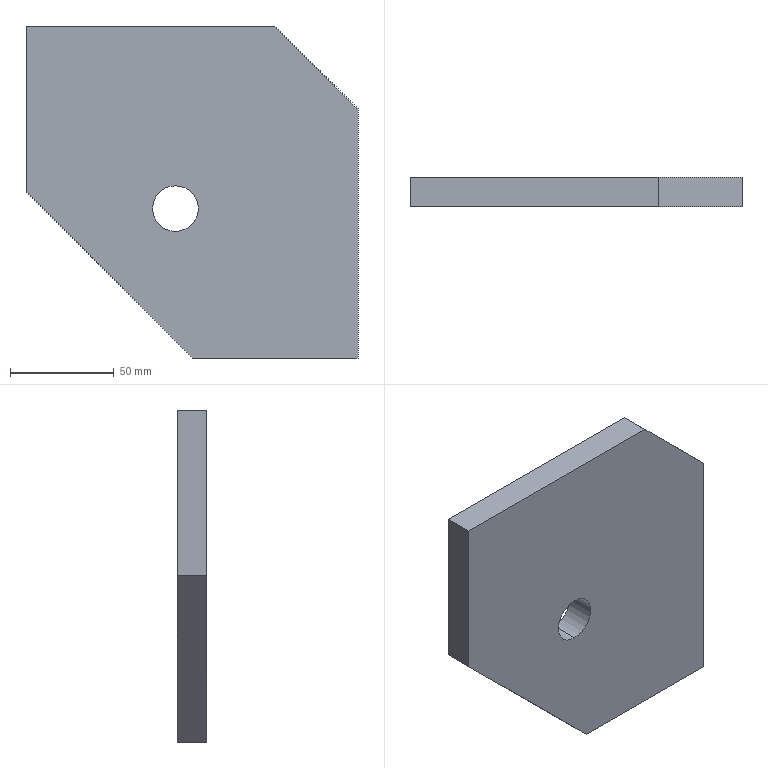Part | SolidWorks | features ICE 2, BaseBody 1 | 1 solid | 10 faces | box 160 x 14 x 160 mm | volume 297078 mm3 | plane 8 | cylinder 2 | commonest cylinder face diameters 22 x2
STEP:
#1=CARTESIAN_POINT('',(-88.,0.,-99.));
#2=VERTEX_POINT('',#1);
#3=CARTESIAN_POINT('',(-88.,0.,-77.));
#4=VERTEX_POINT('',#3);
#5=CARTESIAN_POINT('',(-88.,0.,-88.));
#6=DIRECTION('',(0.,1.,0.));
#7=DIRECTION('',(0.,0.,1.));
#8=AXIS2_PLACEMENT_3D('',#5,#6,#7);
#9=CIRCLE('',#8,11.);
#10=EDGE_CURVE('',#2,#4,#9,.T.);
#11=ORIENTED_EDGE('',*,*,#10,.F.);
#12=CARTESIAN_POINT('',(-88.,14.,-99.));
#13=VERTEX_POINT('',#12);
#14=CARTESIAN_POINT('',(-88.,0.,-99.));
#15=DIRECTION('',(0.,1.,0.));
#16=VECTOR('',#15,1000.);
#17=LINE('',#14,#16);
#18=EDGE_CURVE('',#2,#13,#17,.T.);
#19=ORIENTED_EDGE('',*,*,#18,.T.);
#20=CARTESIAN_POINT('',(-88.,14.,-77.));
#21=VERTEX_POINT('',#20);
#22=CARTESIAN_POINT('',(-88.,14.,-88.));
#23=DIRECTION('',(0.,1.,0.));
#24=DIRECTION('',(0.,0.,1.));
#25=AXIS2_PLACEMENT_3D('',#22,#23,#24);
#26=CIRCLE('',#25,11.);
#27=EDGE_CURVE('',#13,#21,#26,.T.);
#28=ORIENTED_EDGE('',*,*,#27,.T.);
#29=CARTESIAN_POINT('',(-88.,0.,-77.));
#30=DIRECTION('',(0.,1.,0.));
#31=VECTOR('',#30,1000.);
#32=LINE('',#29,#31);
#33=EDGE_CURVE('',#4,#21,#32,.T.);
#34=ORIENTED_EDGE('',*,*,#33,.F.);
#35=EDGE_LOOP('',(#11,#19,#28,#34));
#36=FACE_OUTER_BOUND('',#35,.T.);
#37=CARTESIAN_POINT('',(-88.,0.,-88.));
#38=DIRECTION('',(0.,1.,0.));
#39=DIRECTION('',(0.,0.,1.));
#40=AXIS2_PLACEMENT_3D('',#37,#38,#39);
#41=CYLINDRICAL_SURFACE('',#40,11.);
#42=ADVANCED_FACE('',(#36),#41,.F.);
#43=CARTESIAN_POINT('',(-160.,14.,0.));
#44=VERTEX_POINT('',#43);
#45=CARTESIAN_POINT('',(-160.,14.,-80.));
#46=VERTEX_POINT('',#45);
#47=CARTESIAN_POINT('',(-160.,14.,0.));
#48=DIRECTION('',(0.,0.,-1.));
#49=VECTOR('',#48,1000.);
#50=LINE('',#47,#49);
#51=EDGE_CURVE('',#44,#46,#50,.T.);
#52=ORIENTED_EDGE('',*,*,#51,.F.);
#53=CARTESIAN_POINT('',(-40.,14.,0.));
#54=VERTEX_POINT('',#53);
#55=CARTESIAN_POINT('',(0.,14.,0.));
#56=DIRECTION('',(1.,0.,0.));
#57=VECTOR('',#56,1000.);
#58=LINE('',#55,#57);
#59=EDGE_CURVE('',#44,#54,#58,.T.);
#60=ORIENTED_EDGE('',*,*,#59,.T.);
#61=CARTESIAN_POINT('',(0.,14.,-40.));
#62=VERTEX_POINT('',#61);
#63=CARTESIAN_POINT('',(-40.,14.,0.));
#64=DIRECTION('',(0.7071,0.,-0.7071));
#65=VECTOR('',#64,1000.);
#66=LINE('',#63,#65);
#67=EDGE_CURVE('',#54,#62,#66,.T.);
#68=ORIENTED_EDGE('',*,*,#67,.T.);
#69=CARTESIAN_POINT('',(0.,14.,-160.));
#70=VERTEX_POINT('',#69);
#71=CARTESIAN_POINT('',(0.,14.,0.));
#72=DIRECTION('',(0.,0.,-1.));
#73=VECTOR('',#72,1000.);
#74=LINE('',#71,#73);
#75=EDGE_CURVE('',#62,#70,#74,.T.);
#76=ORIENTED_EDGE('',*,*,#75,.T.);
#77=CARTESIAN_POINT('',(-80.,14.,-160.));
#78=VERTEX_POINT('',#77);
#79=CARTESIAN_POINT('',(0.,14.,-160.));
#80=DIRECTION('',(1.,0.,0.));
#81=VECTOR('',#80,1000.);
#82=LINE('',#79,#81);
#83=EDGE_CURVE('',#78,#70,#82,.T.);
#84=ORIENTED_EDGE('',*,*,#83,.F.);
#85=CARTESIAN_POINT('',(-40.,14.,-200.));
#86=DIRECTION('',(-0.7071,0.,0.7071));
#87=VECTOR('',#86,1000.);
#88=LINE('',#85,#87);
#89=EDGE_CURVE('',#78,#46,#88,.T.);
#90=ORIENTED_EDGE('',*,*,#89,.T.);
#91=EDGE_LOOP('',(#52,#60,#68,#76,#84,#90));
#92=FACE_OUTER_BOUND('',#91,.T.);
#93=CARTESIAN_POINT('',(-88.,14.,-88.));
#94=DIRECTION('',(0.,1.,0.));
#95=DIRECTION('',(0.,0.,1.));
#96=AXIS2_PLACEMENT_3D('',#93,#94,#95);
#97=CIRCLE('',#96,11.);
#98=EDGE_CURVE('',#21,#13,#97,.T.);
#99=ORIENTED_EDGE('',*,*,#98,.F.);
#100=ORIENTED_EDGE('',*,*,#27,.F.);
#101=EDGE_LOOP('',(#99,#100));
#102=FACE_BOUND('',#101,.T.);
#103=CARTESIAN_POINT('',(0.,14.,0.));
#104=DIRECTION('',(0.,1.,0.));
#105=DIRECTION('',(0.,0.,1.));
#106=AXIS2_PLACEMENT_3D('',#103,#104,#105);
#107=PLANE('',#106);
#108=ADVANCED_FACE('',(#92,#102),#107,.T.);
#109=CARTESIAN_POINT('',(0.,0.,-160.));
#110=VERTEX_POINT('',#109);
#111=CARTESIAN_POINT('',(0.,0.,-160.));
#112=DIRECTION('',(0.,1.,0.));
#113=VECTOR('',#112,1000.);
#114=LINE('',#111,#113);
#115=EDGE_CURVE('',#110,#70,#114,.T.);
#116=ORIENTED_EDGE('',*,*,#115,.T.);
#117=ORIENTED_EDGE('',*,*,#75,.F.);
#118=CARTESIAN_POINT('',(0.,0.,-40.));
#119=VERTEX_POINT('',#118);
#120=CARTESIAN_POINT('',(0.,0.,-40.));
#121=DIRECTION('',(0.,-1.,0.));
#122=VECTOR('',#121,1000.);
#123=LINE('',#120,#122);
#124=EDGE_CURVE('',#62,#119,#123,.T.);
#125=ORIENTED_EDGE('',*,*,#124,.T.);
#126=CARTESIAN_POINT('',(0.,0.,-40.));
#127=DIRECTION('',(0.,0.,-1.));
#128=VECTOR('',#127,1000.);
#129=LINE('',#126,#128);
#130=EDGE_CURVE('',#119,#110,#129,.T.);
#131=ORIENTED_EDGE('',*,*,#130,.T.);
#132=EDGE_LOOP('',(#116,#117,#125,#131));
#133=FACE_OUTER_BOUND('',#132,.T.);
#134=CARTESIAN_POINT('',(0.,0.,-40.));
#135=DIRECTION('',(1.,0.,0.));
#136=DIRECTION('',(0.,0.,-1.));
#137=AXIS2_PLACEMENT_3D('',#134,#135,#136);
#138=PLANE('',#137);
#139=ADVANCED_FACE('',(#133),#138,.T.);
#140=CARTESIAN_POINT('',(-40.,0.,0.));
#141=VERTEX_POINT('',#140);
#142=CARTESIAN_POINT('',(-40.,0.,0.));
#143=DIRECTION('',(0.,-1.,0.));
#144=VECTOR('',#143,1000.);
#145=LINE('',#142,#144);
#146=EDGE_CURVE('',#54,#141,#145,.T.);
#147=ORIENTED_EDGE('',*,*,#146,.T.);
#148=CARTESIAN_POINT('',(-40.,0.,0.));
#149=DIRECTION('',(0.7071,0.,-0.7071));
#150=VECTOR('',#149,1000.);
#151=LINE('',#148,#150);
#152=EDGE_CURVE('',#141,#119,#151,.T.);
#153=ORIENTED_EDGE('',*,*,#152,.T.);
#154=ORIENTED_EDGE('',*,*,#124,.F.);
#155=ORIENTED_EDGE('',*,*,#67,.F.);
#156=EDGE_LOOP('',(#147,#153,#154,#155));
#157=FACE_OUTER_BOUND('',#156,.T.);
#158=CARTESIAN_POINT('',(-40.,0.,0.));
#159=DIRECTION('',(0.7071,0.,0.7071));
#160=DIRECTION('',(0.7071,0.,-0.7071));
#161=AXIS2_PLACEMENT_3D('',#158,#159,#160);
#162=PLANE('',#161);
#163=ADVANCED_FACE('',(#157),#162,.T.);
#164=CARTESIAN_POINT('',(-160.,0.,0.));
#165=VERTEX_POINT('',#164);
#166=CARTESIAN_POINT('',(-160.,0.,0.));
#167=DIRECTION('',(0.,1.,0.));
#168=VECTOR('',#167,1000.);
#169=LINE('',#166,#168);
#170=EDGE_CURVE('',#165,#44,#169,.T.);
#171=ORIENTED_EDGE('',*,*,#170,.F.);
#172=CARTESIAN_POINT('',(-200.,0.,0.));
#173=DIRECTION('',(1.,0.,0.));
#174=VECTOR('',#173,1000.);
#175=LINE('',#172,#174);
#176=EDGE_CURVE('',#165,#141,#175,.T.);
#177=ORIENTED_EDGE('',*,*,#176,.T.);
#178=ORIENTED_EDGE('',*,*,#146,.F.);
#179=ORIENTED_EDGE('',*,*,#59,.F.);
#180=EDGE_LOOP('',(#171,#177,#178,#179));
#181=FACE_OUTER_BOUND('',#180,.T.);
#182=CARTESIAN_POINT('',(-200.,0.,0.));
#183=DIRECTION('',(0.,0.,1.));
#184=DIRECTION('',(1.,0.,0.));
#185=AXIS2_PLACEMENT_3D('',#182,#183,#184);
#186=PLANE('',#185);
#187=ADVANCED_FACE('',(#181),#186,.T.);
#188=CARTESIAN_POINT('',(-160.,0.,-80.));
#189=VERTEX_POINT('',#188);
#190=CARTESIAN_POINT('',(-160.,0.,-80.));
#191=DIRECTION('',(0.,-1.,0.));
#192=VECTOR('',#191,1000.);
#193=LINE('',#190,#192);
#194=EDGE_CURVE('',#46,#189,#193,.T.);
#195=ORIENTED_EDGE('',*,*,#194,.F.);
#196=ORIENTED_EDGE('',*,*,#89,.F.);
#197=CARTESIAN_POINT('',(-80.,0.,-160.));
#198=VERTEX_POINT('',#197);
#199=CARTESIAN_POINT('',(-80.,0.,-160.));
#200=DIRECTION('',(0.,1.,0.));
#201=VECTOR('',#200,1000.);
#202=LINE('',#199,#201);
#203=EDGE_CURVE('',#198,#78,#202,.T.);
#204=ORIENTED_EDGE('',*,*,#203,.F.);
#205=CARTESIAN_POINT('',(-40.,0.,-200.));
#206=DIRECTION('',(-0.7071,0.,0.7071));
#207=VECTOR('',#206,1000.);
#208=LINE('',#205,#207);
#209=EDGE_CURVE('',#198,#189,#208,.T.);
#210=ORIENTED_EDGE('',*,*,#209,.T.);
#211=EDGE_LOOP('',(#195,#196,#204,#210));
#212=FACE_OUTER_BOUND('',#211,.T.);
#213=CARTESIAN_POINT('',(-40.,0.,-200.));
#214=DIRECTION('',(-0.7071,0.,-0.7071));
#215=DIRECTION('',(-0.7071,0.,0.7071));
#216=AXIS2_PLACEMENT_3D('',#213,#214,#215);
#217=PLANE('',#216);
#218=ADVANCED_FACE('',(#212),#217,.T.);
#219=ORIENTED_EDGE('',*,*,#176,.F.);
#220=CARTESIAN_POINT('',(-160.,0.,0.));
#221=DIRECTION('',(0.,0.,-1.));
#222=VECTOR('',#221,1000.);
#223=LINE('',#220,#222);
#224=EDGE_CURVE('',#165,#189,#223,.T.);
#225=ORIENTED_EDGE('',*,*,#224,.T.);
#226=ORIENTED_EDGE('',*,*,#209,.F.);
#227=CARTESIAN_POINT('',(0.,0.,-160.));
#228=DIRECTION('',(1.,0.,0.));
#229=VECTOR('',#228,1000.);
#230=LINE('',#227,#229);
#231=EDGE_CURVE('',#198,#110,#230,.T.);
#232=ORIENTED_EDGE('',*,*,#231,.T.);
#233=ORIENTED_EDGE('',*,*,#130,.F.);
#234=ORIENTED_EDGE('',*,*,#152,.F.);
#235=EDGE_LOOP('',(#219,#225,#226,#232,#233,#234));
#236=FACE_OUTER_BOUND('',#235,.T.);
#237=CARTESIAN_POINT('',(-88.,0.,-88.));
#238=DIRECTION('',(0.,1.,0.));
#239=DIRECTION('',(0.,0.,1.));
#240=AXIS2_PLACEMENT_3D('',#237,#238,#239);
#241=CIRCLE('',#240,11.);
#242=EDGE_CURVE('',#4,#2,#241,.T.);
#243=ORIENTED_EDGE('',*,*,#242,.T.);
#244=ORIENTED_EDGE('',*,*,#10,.T.);
#245=EDGE_LOOP('',(#243,#244));
#246=FACE_BOUND('',#245,.T.);
#247=CARTESIAN_POINT('',(0.,0.,0.));
#248=DIRECTION('',(0.,1.,0.));
#249=DIRECTION('',(0.,0.,1.));
#250=AXIS2_PLACEMENT_3D('',#247,#248,#249);
#251=PLANE('',#250);
#252=ADVANCED_FACE('',(#236,#246),#251,.F.);
#253=ORIENTED_EDGE('',*,*,#18,.F.);
#254=ORIENTED_EDGE('',*,*,#242,.F.);
#255=ORIENTED_EDGE('',*,*,#33,.T.);
#256=ORIENTED_EDGE('',*,*,#98,.T.);
#257=EDGE_LOOP('',(#253,#254,#255,#256));
#258=FACE_OUTER_BOUND('',#257,.T.);
#259=CARTESIAN_POINT('',(-88.,0.,-88.));
#260=DIRECTION('',(0.,1.,0.));
#261=DIRECTION('',(0.,0.,1.));
#262=AXIS2_PLACEMENT_3D('',#259,#260,#261);
#263=CYLINDRICAL_SURFACE('',#262,11.);
#264=ADVANCED_FACE('',(#258),#263,.F.);
#265=ORIENTED_EDGE('',*,*,#203,.T.);
#266=ORIENTED_EDGE('',*,*,#83,.T.);
#267=ORIENTED_EDGE('',*,*,#115,.F.);
#268=ORIENTED_EDGE('',*,*,#231,.F.);
#269=EDGE_LOOP('',(#265,#266,#267,#268));
#270=FACE_OUTER_BOUND('',#269,.T.);
#271=CARTESIAN_POINT('',(0.,0.,-160.));
#272=DIRECTION('',(0.,0.,1.));
#273=DIRECTION('',(1.,0.,0.));
#274=AXIS2_PLACEMENT_3D('',#271,#272,#273);
#275=PLANE('',#274);
#276=ADVANCED_FACE('',(#270),#275,.F.);
#277=ORIENTED_EDGE('',*,*,#194,.T.);
#278=ORIENTED_EDGE('',*,*,#224,.F.);
#279=ORIENTED_EDGE('',*,*,#170,.T.);
#280=ORIENTED_EDGE('',*,*,#51,.T.);
#281=EDGE_LOOP('',(#277,#278,#279,#280));
#282=FACE_OUTER_BOUND('',#281,.T.);
#283=CARTESIAN_POINT('',(-160.,0.,0.));
#284=DIRECTION('',(1.,0.,0.));
#285=DIRECTION('',(0.,0.,-1.));
#286=AXIS2_PLACEMENT_3D('',#283,#284,#285);
#287=PLANE('',#286);
#288=ADVANCED_FACE('',(#282),#287,.F.);
#289=CLOSED_SHELL('',(#42,#108,#139,#163,#187,#218,#252,#264,#276,#288));
#290=MANIFOLD_SOLID_BREP('',#289);
#291=CARTESIAN_POINT('',(0.,0.,0.));
#292=DIRECTION('',(0.,0.,1.));
#293=DIRECTION('',(1.,0.,0.));
#294=AXIS2_PLACEMENT_3D('',#291,#292,#293);
#295=(LENGTH_UNIT()NAMED_UNIT(*)SI_UNIT(.MILLI.,.METRE.));
#296=UNCERTAINTY_MEASURE_WITH_UNIT(LENGTH_MEASURE(0.00001),#295,'','');
#297=(NAMED_UNIT(*)PLANE_ANGLE_UNIT()SI_UNIT($,.RADIAN.));
#298=(NAMED_UNIT(*)SI_UNIT($,.STERADIAN.)SOLID_ANGLE_UNIT());
#299=(GEOMETRIC_REPRESENTATION_CONTEXT(3)GLOBAL_UNCERTAINTY_ASSIGNED_CONTEXT((#296))GLOBAL_UNIT_ASSIGNED_CONTEXT((#295,#297,#298))REPRESENTATION_CONTEXT('',''));
#300=ADVANCED_BREP_SHAPE_REPRESENTATION('',(#290,#294),#299);